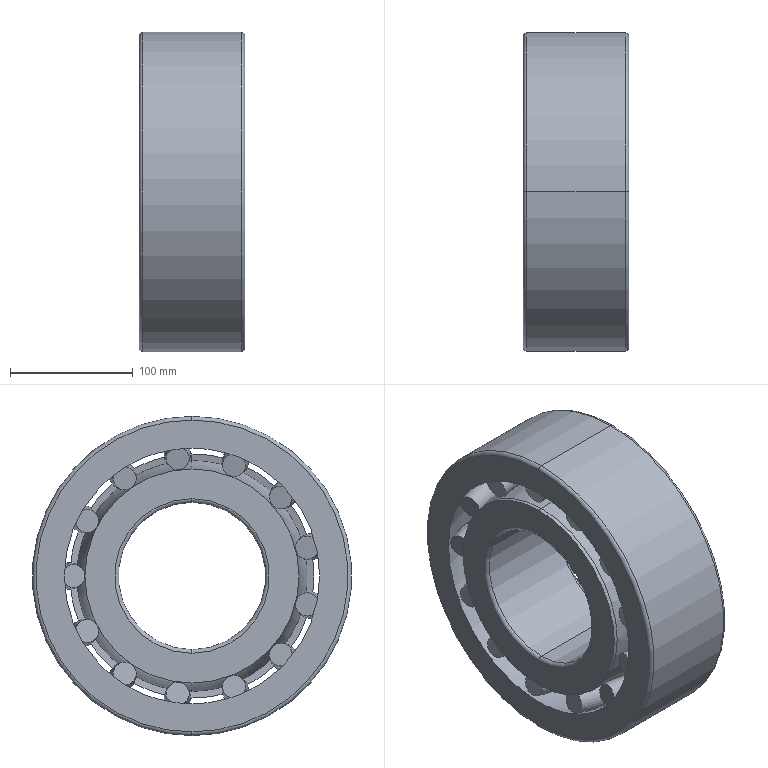Part | STEP file | GB/T288-94 spherical roller bearing 22324C_1 | 1 solid | 160 faces | box 86 x 260 x 260 mm | volume 2801542 mm3 | plane 56 | other 52 | cone 28 | torus 16 | cylinder 6 | sphere 2 | commonest cylinder face diameters 120 x2 198.75 x2 260 x2